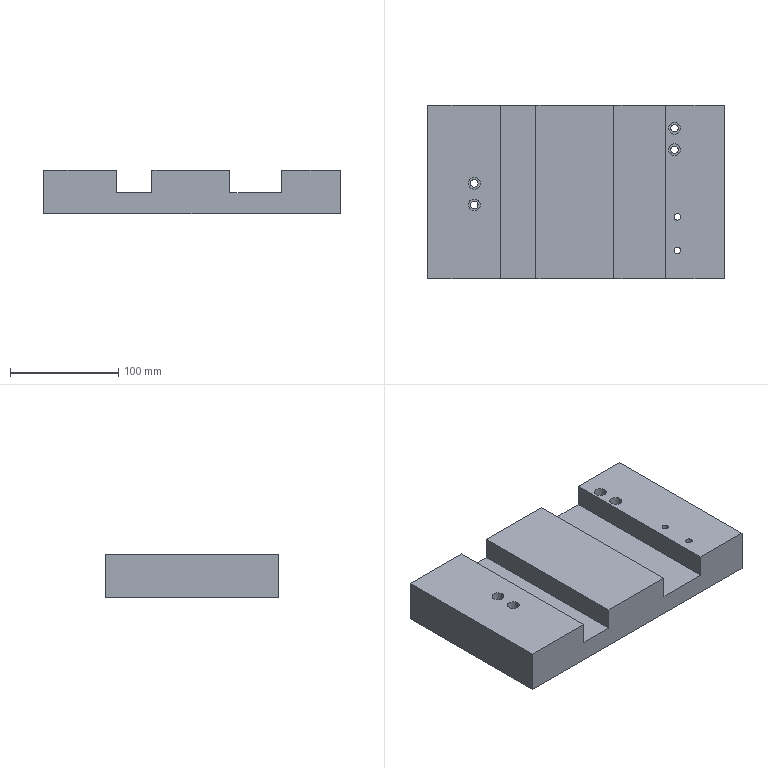Part | 1 solid | 38 faces | box 273.935 x 160 x 40 mm | volume 1476976 mm3 | cylinder 20 | plane 18 | commonest cylinder face diameters 7 x8 11 x8 6 x4